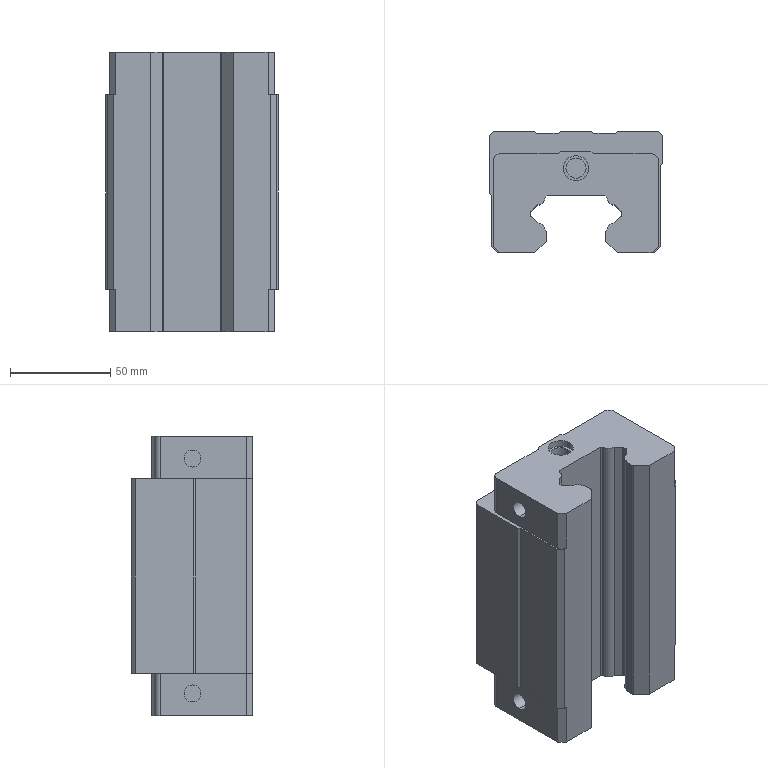Part | SolidWorks | features BaseBody 1 | 1 solid | 122 faces | box 86 x 60.5 x 139.4 mm | volume 512577 mm3 | plane 74 | cylinder 48 | commonest cylinder face diameters 10 x12 8.5 x8 1 x4 1.6 x4 2.4 x4 6 x4